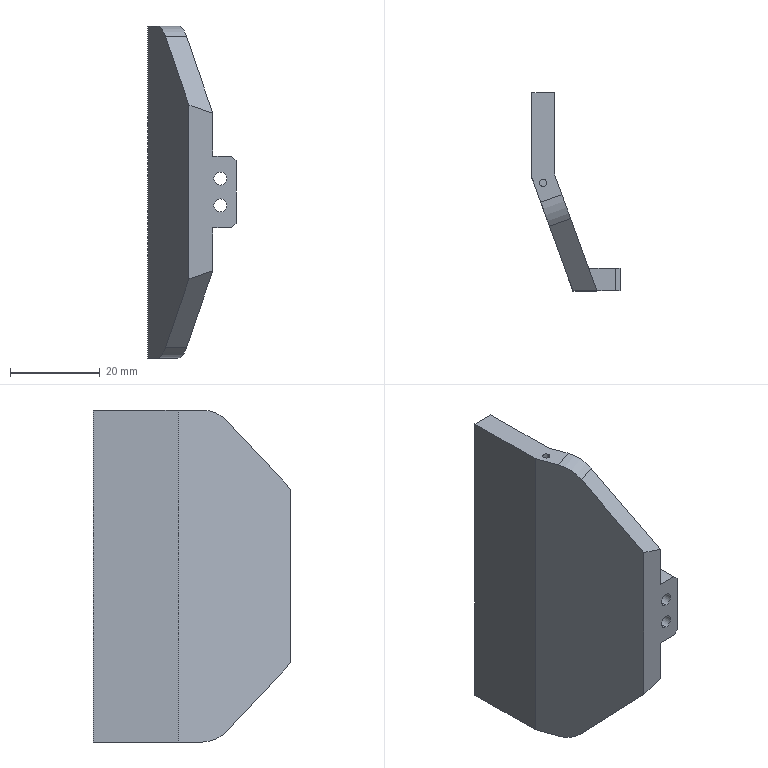NC program | NX | posted with a generic post | part box 19.643 x 44.061 x 74 mm
Whole program:
N10 G17 G21 G94 G90
(PLANAR_MILL_2 , TOOL : D8开粗)
N12 T02 M6
N14 G54
N16 G17 G0 G90 X42. Y0. B0. C0. S3500 M3
N18 G43 Z30. H2
N20 Z2.05
N22 G94 G1 Z0.05 F800.
N24 X36.
N26 X32.
N28 X26.
N30 Z2.05
N32 G0 Z30.
N34 X-26.
N36 Z2.05
N38 G1 Z0.05
N40 X-32.
N42 X-36.
N44 X-42.
N46 Z2.05
N48 G0 Z30.
N50 M5
(PLANAR_MILL_2_COPY_COPY , TOOL : D8精光)
N52 T03 M6
N54 G54
N56 G17 G0 G90 X42. Y0. B0. C0. S3500 M3
N58 G43 Z30. H3
N60 Z2.
N62 G94 G1 Z0. F800.
N64 X36.
N66 X32.
N68 X26.
N70 Z2.
N72 G0 Z30.
N74 X-26.
N76 Z2.
N78 G1 Z0.
N80 X-32.
N82 X-36.
N84 X-42.
N86 Z2.
N88 G0 Z30.
N90 M5
(PLANAR_MILL_3 , TOOL : D4点钻)
N92 T05 M6
N94 G54
N96 G17 G0 G90 X-37.55 Y-5. B0. C0. S3500 M3
N98 G43 Z30. H5
N100 Z0.5
N102 G94 G1 Z-1.5 F800.
N104 Y-2.5
N106 Y2.5
N108 Y5.
N110 Z0.5
N112 G0 Z30.
N114 X-30.45
N116 Z0.5
N118 G1 Z-1.5
N120 Y2.5
N122 Y-2.5
N124 Y-5.
N126 Z0.5
N128 G0 Z30.
N130 X30.45
N132 Z0.5
N134 G1 Z-1.5
N136 Y-2.5
N138 Y2.5
N140 Y5.
N142 Z0.5
N144 G0 Z30.
N146 X37.55
N148 Z0.5
N150 G1 Z-1.5
N152 Y2.5
N154 Y-2.5
N156 Y-5.
N158 Z0.5
N160 G0 Z30.
(PLANAR_MILL_3_COPY , TOOL : D4点钻)
N162 X-37.5 S4500
N164 Z0.5
N166 G1 Z-1.5 F600.
N168 Y-2.5
N170 Y2.5
N172 Y5.
N174 Z0.5
N176 G0 Z30.
N178 X-30.5
N180 Z0.5
N182 G1 Z-1.5
N184 Y2.5
N186 Y-2.5
N188 Y-5.
N190 Z0.5
N192 G0 Z30.
N194 X30.5
N196 Z0.5
N198 G1 Z-1.5
N200 Y-2.5
N202 Y2.5
N204 Y5.
N206 Z0.5
N208 G0 Z30.
N210 X37.5
N212 Z0.5
N214 G1 Z-1.5
N216 Y2.5
N218 Y-2.5
N220 Y-5.
N222 Z0.5
N224 G0 Z30.
(DRILLING , TOOL : D4点钻)
N226 X-34. Y0. S3000
N228 G81 G98 Z-1.3 F200. R3.
N230 X34.
N232 G80
N234 G0 X34. Y0. Z30.
N236 M5
(DRILLING_COPY , TOOL : D2.3钻头)
N238 T06 M6
N240 G54
N242 G17 G0 G90 X-34. Y0. B0. C0. S3000 M3
N244 G43 Z30. H6
N246 G94 G81 G98 Z-7. F150. R3.
N248 X34.
N250 G80
N252 G0 X34. Y0. Z30.
N254 M5
N256 M2